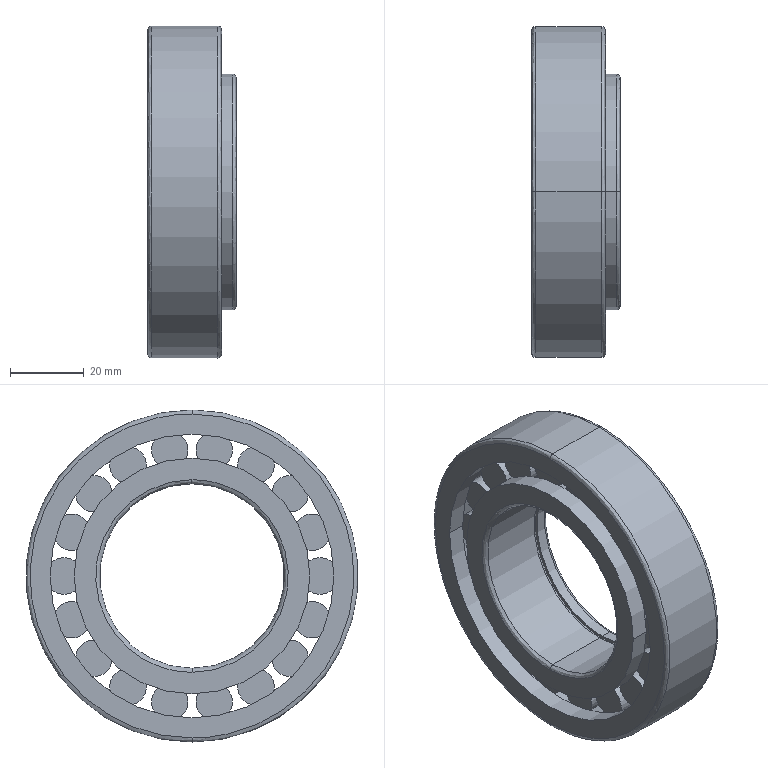Part | SolidWorks | features BaseBody 20 | 20 solids | 111 faces | box 24 x 90 x 90 mm | volume 70515 mm3 | cylinder 54 | plane 45 | spline 12 | commonest cylinder face diameters 9.913 x32 9.912 x4 50 x4 63.9 x4 76.905 x4 59.5 x2